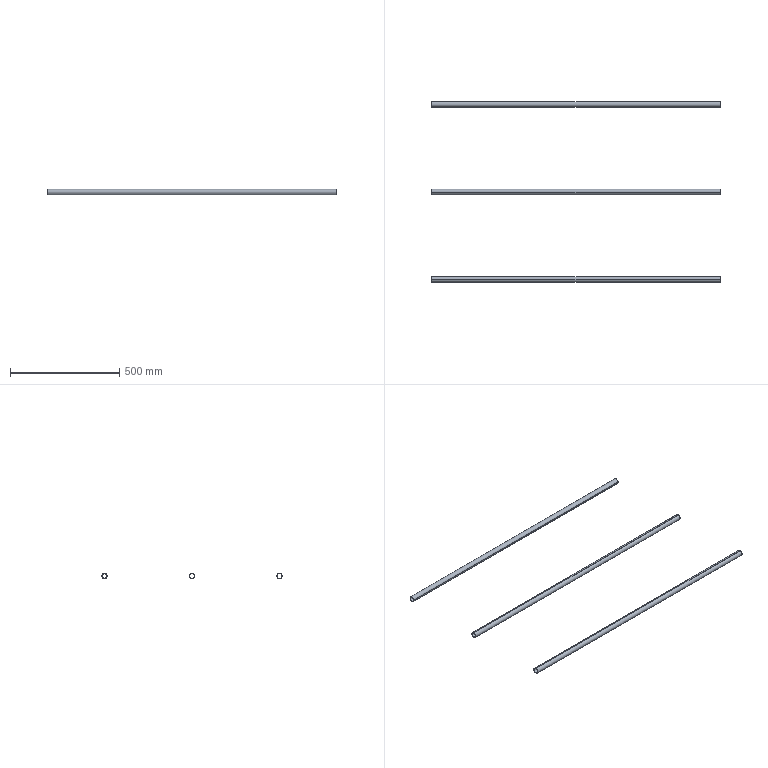Part | STEP file | 电柜护栏3栏杆_Default<As Machined> | 3 solids | 18 faces | box 1320 x 825 x 25 mm | volume 438535 mm3 | cylinder 12 | plane 6 | commonest cylinder face diameters 22 x6 25 x6
STEP:
#1=CARTESIAN_POINT('',(0.,0.,0.));
#2=DIRECTION('',(0.,0.,1.));
#3=DIRECTION('',(1.,0.,0.));
#4=AXIS2_PLACEMENT_3D('',#1,#2,#3);
#5=CARTESIAN_POINT('',(-1320.,0.,12.5));
#6=VERTEX_POINT('',#5);
#7=CARTESIAN_POINT('',(-1320.,0.,-12.5));
#8=VERTEX_POINT('',#7);
#9=CARTESIAN_POINT('',(-1320.,0.,0.));
#10=DIRECTION('',(-1.,0.,0.));
#11=DIRECTION('',(0.,-1.,0.));
#12=AXIS2_PLACEMENT_3D('',#9,#10,#11);
#13=CIRCLE('',#12,12.5);
#14=CARTESIAN_POINT('',(-1320.,0.,0.));
#15=DIRECTION('',(1.,0.,0.));
#16=DIRECTION('',(0.,0.,-1.));
#17=AXIS2_PLACEMENT_3D('',#14,#15,#16);
#18=CYLINDRICAL_SURFACE('',#17,12.5);
#19=CARTESIAN_POINT('',(4.712,0.));
#20=DIRECTION('',(-1.,0.));
#21=VECTOR('',#20,1.);
#22=LINE('',#19,#21);
#23=(GEOMETRIC_REPRESENTATION_CONTEXT(2)PARAMETRIC_REPRESENTATION_CONTEXT()REPRESENTATION_CONTEXT('',''));
#24=DEFINITIONAL_REPRESENTATION('',(#22),#23);
#25=PCURVE('',#18,#24);
#26=CARTESIAN_POINT('',(-1320.,0.,0.));
#27=DIRECTION('',(-1.,0.,0.));
#28=DIRECTION('',(0.,-1.,0.));
#29=AXIS2_PLACEMENT_3D('',#26,#27,#28);
#30=PLANE('',#29);
#31=CARTESIAN_POINT('',(0.,0.));
#32=DIRECTION('',(1.,0.));
#33=AXIS2_PLACEMENT_2D('',#31,#32);
#34=CIRCLE('',#33,12.5);
#35=(GEOMETRIC_REPRESENTATION_CONTEXT(2)PARAMETRIC_REPRESENTATION_CONTEXT()REPRESENTATION_CONTEXT('',''));
#36=DEFINITIONAL_REPRESENTATION('',(#34),#35);
#37=PCURVE('',#30,#36);
#38=SURFACE_CURVE('',#13,(#25,#37),.PCURVE_S1.);
#39=EDGE_CURVE('',#6,#8,#38,.T.);
#40=ORIENTED_EDGE('',*,*,#39,.F.);
#41=CARTESIAN_POINT('',(0.,0.,12.5));
#42=VERTEX_POINT('',#41);
#43=CARTESIAN_POINT('',(-1320.,0.,12.5));
#44=DIRECTION('',(1.,0.,0.));
#45=VECTOR('',#44,1.);
#46=LINE('',#43,#45);
#47=CARTESIAN_POINT('',(3.142,0.));
#48=DIRECTION('',(0.,1.));
#49=VECTOR('',#48,1.);
#50=LINE('',#47,#49);
#51=(GEOMETRIC_REPRESENTATION_CONTEXT(2)PARAMETRIC_REPRESENTATION_CONTEXT()REPRESENTATION_CONTEXT('',''));
#52=DEFINITIONAL_REPRESENTATION('',(#50),#51);
#53=PCURVE('',#18,#52);
#54=CARTESIAN_POINT('',(-1320.,0.,0.));
#55=DIRECTION('',(1.,0.,0.));
#56=DIRECTION('',(0.,0.,-1.));
#57=AXIS2_PLACEMENT_3D('',#54,#55,#56);
#58=CYLINDRICAL_SURFACE('',#57,12.5);
#59=CARTESIAN_POINT('',(3.142,0.));
#60=DIRECTION('',(0.,1.));
#61=VECTOR('',#60,1.);
#62=LINE('',#59,#61);
#63=(GEOMETRIC_REPRESENTATION_CONTEXT(2)PARAMETRIC_REPRESENTATION_CONTEXT()REPRESENTATION_CONTEXT('',''));
#64=DEFINITIONAL_REPRESENTATION('',(#62),#63);
#65=PCURVE('',#58,#64);
#66=SURFACE_CURVE('',#46,(#53,#65),.PCURVE_S1.);
#67=EDGE_CURVE('',#6,#42,#66,.T.);
#68=ORIENTED_EDGE('',*,*,#67,.T.);
#69=CARTESIAN_POINT('',(0.,0.,-12.5));
#70=VERTEX_POINT('',#69);
#71=CARTESIAN_POINT('',(0.,0.,0.));
#72=DIRECTION('',(-1.,0.,0.));
#73=DIRECTION('',(0.,-1.,0.));
#74=AXIS2_PLACEMENT_3D('',#71,#72,#73);
#75=CIRCLE('',#74,12.5);
#76=CARTESIAN_POINT('',(4.712,1320.));
#77=DIRECTION('',(-1.,0.));
#78=VECTOR('',#77,1.);
#79=LINE('',#76,#78);
#80=(GEOMETRIC_REPRESENTATION_CONTEXT(2)PARAMETRIC_REPRESENTATION_CONTEXT()REPRESENTATION_CONTEXT('',''));
#81=DEFINITIONAL_REPRESENTATION('',(#79),#80);
#82=PCURVE('',#18,#81);
#83=CARTESIAN_POINT('',(0.,0.,0.));
#84=DIRECTION('',(-1.,0.,0.));
#85=DIRECTION('',(0.,-1.,0.));
#86=AXIS2_PLACEMENT_3D('',#83,#84,#85);
#87=PLANE('',#86);
#88=CARTESIAN_POINT('',(0.,0.));
#89=DIRECTION('',(1.,0.));
#90=AXIS2_PLACEMENT_2D('',#88,#89);
#91=CIRCLE('',#90,12.5);
#92=(GEOMETRIC_REPRESENTATION_CONTEXT(2)PARAMETRIC_REPRESENTATION_CONTEXT()REPRESENTATION_CONTEXT('',''));
#93=DEFINITIONAL_REPRESENTATION('',(#91),#92);
#94=PCURVE('',#87,#93);
#95=SURFACE_CURVE('',#75,(#82,#94),.PCURVE_S1.);
#96=EDGE_CURVE('',#42,#70,#95,.T.);
#97=ORIENTED_EDGE('',*,*,#96,.T.);
#98=CARTESIAN_POINT('',(-1320.,0.,-12.5));
#99=DIRECTION('',(1.,0.,0.));
#100=VECTOR('',#99,1.);
#101=LINE('',#98,#100);
#102=CARTESIAN_POINT('',(0.,0.));
#103=DIRECTION('',(0.,1.));
#104=VECTOR('',#103,1.);
#105=LINE('',#102,#104);
#106=(GEOMETRIC_REPRESENTATION_CONTEXT(2)PARAMETRIC_REPRESENTATION_CONTEXT()REPRESENTATION_CONTEXT('',''));
#107=DEFINITIONAL_REPRESENTATION('',(#105),#106);
#108=PCURVE('',#18,#107);
#109=CARTESIAN_POINT('',(6.283,0.));
#110=DIRECTION('',(0.,1.));
#111=VECTOR('',#110,1.);
#112=LINE('',#109,#111);
#113=(GEOMETRIC_REPRESENTATION_CONTEXT(2)PARAMETRIC_REPRESENTATION_CONTEXT()REPRESENTATION_CONTEXT('',''));
#114=DEFINITIONAL_REPRESENTATION('',(#112),#113);
#115=PCURVE('',#58,#114);
#116=SURFACE_CURVE('',#101,(#108,#115),.PCURVE_S1.);
#117=EDGE_CURVE('',#8,#70,#116,.T.);
#118=ORIENTED_EDGE('',*,*,#117,.F.);
#119=EDGE_LOOP('',(#40,#68,#97,#118));
#120=FACE_BOUND('',#119,.T.);
#121=ADVANCED_FACE('',(#120),#18,.T.);
#122=CARTESIAN_POINT('',(-1320.,0.,-11.));
#123=VERTEX_POINT('',#122);
#124=CARTESIAN_POINT('',(0.,0.,-11.));
#125=VERTEX_POINT('',#124);
#126=CARTESIAN_POINT('',(-1320.,0.,-11.));
#127=DIRECTION('',(1.,0.,0.));
#128=VECTOR('',#127,1.);
#129=LINE('',#126,#128);
#130=CARTESIAN_POINT('',(-1320.,0.,0.));
#131=DIRECTION('',(1.,0.,0.));
#132=DIRECTION('',(0.,0.,-1.));
#133=AXIS2_PLACEMENT_3D('',#130,#131,#132);
#134=CYLINDRICAL_SURFACE('',#133,11.);
#135=CARTESIAN_POINT('',(6.283,0.));
#136=DIRECTION('',(0.,1.));
#137=VECTOR('',#136,1.);
#138=LINE('',#135,#137);
#139=(GEOMETRIC_REPRESENTATION_CONTEXT(2)PARAMETRIC_REPRESENTATION_CONTEXT()REPRESENTATION_CONTEXT('',''));
#140=DEFINITIONAL_REPRESENTATION('',(#138),#139);
#141=PCURVE('',#134,#140);
#142=CARTESIAN_POINT('',(-1320.,0.,0.));
#143=DIRECTION('',(1.,0.,0.));
#144=DIRECTION('',(0.,0.,-1.));
#145=AXIS2_PLACEMENT_3D('',#142,#143,#144);
#146=CYLINDRICAL_SURFACE('',#145,11.);
#147=CARTESIAN_POINT('',(0.,0.));
#148=DIRECTION('',(0.,1.));
#149=VECTOR('',#148,1.);
#150=LINE('',#147,#149);
#151=(GEOMETRIC_REPRESENTATION_CONTEXT(2)PARAMETRIC_REPRESENTATION_CONTEXT()REPRESENTATION_CONTEXT('',''));
#152=DEFINITIONAL_REPRESENTATION('',(#150),#151);
#153=PCURVE('',#146,#152);
#154=SURFACE_CURVE('',#129,(#141,#153),.PCURVE_S1.);
#155=EDGE_CURVE('',#123,#125,#154,.T.);
#156=ORIENTED_EDGE('',*,*,#155,.T.);
#157=CARTESIAN_POINT('',(0.,0.,11.));
#158=VERTEX_POINT('',#157);
#159=CARTESIAN_POINT('',(0.,0.,0.));
#160=DIRECTION('',(-1.,0.,0.));
#161=DIRECTION('',(0.,-1.,0.));
#162=AXIS2_PLACEMENT_3D('',#159,#160,#161);
#163=CIRCLE('',#162,11.);
#164=CARTESIAN_POINT('',(10.996,1320.));
#165=DIRECTION('',(-1.,0.));
#166=VECTOR('',#165,1.);
#167=LINE('',#164,#166);
#168=(GEOMETRIC_REPRESENTATION_CONTEXT(2)PARAMETRIC_REPRESENTATION_CONTEXT()REPRESENTATION_CONTEXT('',''));
#169=DEFINITIONAL_REPRESENTATION('',(#167),#168);
#170=PCURVE('',#134,#169);
#171=CARTESIAN_POINT('',(0.,0.));
#172=DIRECTION('',(1.,0.));
#173=AXIS2_PLACEMENT_2D('',#171,#172);
#174=CIRCLE('',#173,11.);
#175=(GEOMETRIC_REPRESENTATION_CONTEXT(2)PARAMETRIC_REPRESENTATION_CONTEXT()REPRESENTATION_CONTEXT('',''));
#176=DEFINITIONAL_REPRESENTATION('',(#174),#175);
#177=PCURVE('',#87,#176);
#178=SURFACE_CURVE('',#163,(#170,#177),.PCURVE_S1.);
#179=EDGE_CURVE('',#125,#158,#178,.T.);
#180=ORIENTED_EDGE('',*,*,#179,.T.);
#181=CARTESIAN_POINT('',(-1320.,0.,11.));
#182=VERTEX_POINT('',#181);
#183=CARTESIAN_POINT('',(-1320.,0.,11.));
#184=DIRECTION('',(1.,0.,0.));
#185=VECTOR('',#184,1.);
#186=LINE('',#183,#185);
#187=CARTESIAN_POINT('',(3.142,0.));
#188=DIRECTION('',(0.,1.));
#189=VECTOR('',#188,1.);
#190=LINE('',#187,#189);
#191=(GEOMETRIC_REPRESENTATION_CONTEXT(2)PARAMETRIC_REPRESENTATION_CONTEXT()REPRESENTATION_CONTEXT('',''));
#192=DEFINITIONAL_REPRESENTATION('',(#190),#191);
#193=PCURVE('',#134,#192);
#194=CARTESIAN_POINT('',(3.142,0.));
#195=DIRECTION('',(0.,1.));
#196=VECTOR('',#195,1.);
#197=LINE('',#194,#196);
#198=(GEOMETRIC_REPRESENTATION_CONTEXT(2)PARAMETRIC_REPRESENTATION_CONTEXT()REPRESENTATION_CONTEXT('',''));
#199=DEFINITIONAL_REPRESENTATION('',(#197),#198);
#200=PCURVE('',#146,#199);
#201=SURFACE_CURVE('',#186,(#193,#200),.PCURVE_S1.);
#202=EDGE_CURVE('',#182,#158,#201,.T.);
#203=ORIENTED_EDGE('',*,*,#202,.F.);
#204=CARTESIAN_POINT('',(-1320.,0.,0.));
#205=DIRECTION('',(-1.,0.,0.));
#206=DIRECTION('',(0.,-1.,0.));
#207=AXIS2_PLACEMENT_3D('',#204,#205,#206);
#208=CIRCLE('',#207,11.);
#209=CARTESIAN_POINT('',(10.996,0.));
#210=DIRECTION('',(-1.,0.));
#211=VECTOR('',#210,1.);
#212=LINE('',#209,#211);
#213=(GEOMETRIC_REPRESENTATION_CONTEXT(2)PARAMETRIC_REPRESENTATION_CONTEXT()REPRESENTATION_CONTEXT('',''));
#214=DEFINITIONAL_REPRESENTATION('',(#212),#213);
#215=PCURVE('',#134,#214);
#216=CARTESIAN_POINT('',(0.,0.));
#217=DIRECTION('',(1.,0.));
#218=AXIS2_PLACEMENT_2D('',#216,#217);
#219=CIRCLE('',#218,11.);
#220=(GEOMETRIC_REPRESENTATION_CONTEXT(2)PARAMETRIC_REPRESENTATION_CONTEXT()REPRESENTATION_CONTEXT('',''));
#221=DEFINITIONAL_REPRESENTATION('',(#219),#220);
#222=PCURVE('',#30,#221);
#223=SURFACE_CURVE('',#208,(#215,#222),.PCURVE_S1.);
#224=EDGE_CURVE('',#123,#182,#223,.T.);
#225=ORIENTED_EDGE('',*,*,#224,.F.);
#226=EDGE_LOOP('',(#156,#180,#203,#225));
#227=FACE_BOUND('',#226,.F.);
#228=ADVANCED_FACE('',(#227),#134,.F.);
#229=CARTESIAN_POINT('',(0.,0.,0.));
#230=DIRECTION('',(-1.,0.,0.));
#231=DIRECTION('',(0.,-1.,0.));
#232=AXIS2_PLACEMENT_3D('',#229,#230,#231);
#233=CIRCLE('',#232,11.);
#234=CARTESIAN_POINT('',(4.712,1320.));
#235=DIRECTION('',(-1.,0.));
#236=VECTOR('',#235,1.);
#237=LINE('',#234,#236);
#238=(GEOMETRIC_REPRESENTATION_CONTEXT(2)PARAMETRIC_REPRESENTATION_CONTEXT()REPRESENTATION_CONTEXT('',''));
#239=DEFINITIONAL_REPRESENTATION('',(#237),#238);
#240=PCURVE('',#146,#239);
#241=CARTESIAN_POINT('',(0.,0.));
#242=DIRECTION('',(1.,0.));
#243=AXIS2_PLACEMENT_2D('',#241,#242);
#244=CIRCLE('',#243,11.);
#245=(GEOMETRIC_REPRESENTATION_CONTEXT(2)PARAMETRIC_REPRESENTATION_CONTEXT()REPRESENTATION_CONTEXT('',''));
#246=DEFINITIONAL_REPRESENTATION('',(#244),#245);
#247=PCURVE('',#87,#246);
#248=SURFACE_CURVE('',#233,(#240,#247),.PCURVE_S1.);
#249=EDGE_CURVE('',#158,#125,#248,.T.);
#250=ORIENTED_EDGE('',*,*,#249,.T.);
#251=ORIENTED_EDGE('',*,*,#155,.F.);
#252=CARTESIAN_POINT('',(-1320.,0.,0.));
#253=DIRECTION('',(-1.,0.,0.));
#254=DIRECTION('',(0.,-1.,0.));
#255=AXIS2_PLACEMENT_3D('',#252,#253,#254);
#256=CIRCLE('',#255,11.);
#257=CARTESIAN_POINT('',(4.712,0.));
#258=DIRECTION('',(-1.,0.));
#259=VECTOR('',#258,1.);
#260=LINE('',#257,#259);
#261=(GEOMETRIC_REPRESENTATION_CONTEXT(2)PARAMETRIC_REPRESENTATION_CONTEXT()REPRESENTATION_CONTEXT('',''));
#262=DEFINITIONAL_REPRESENTATION('',(#260),#261);
#263=PCURVE('',#146,#262);
#264=CARTESIAN_POINT('',(0.,0.));
#265=DIRECTION('',(1.,0.));
#266=AXIS2_PLACEMENT_2D('',#264,#265);
#267=CIRCLE('',#266,11.);
#268=(GEOMETRIC_REPRESENTATION_CONTEXT(2)PARAMETRIC_REPRESENTATION_CONTEXT()REPRESENTATION_CONTEXT('',''));
#269=DEFINITIONAL_REPRESENTATION('',(#267),#268);
#270=PCURVE('',#30,#269);
#271=SURFACE_CURVE('',#256,(#263,#270),.PCURVE_S1.);
#272=EDGE_CURVE('',#182,#123,#271,.T.);
#273=ORIENTED_EDGE('',*,*,#272,.F.);
#274=ORIENTED_EDGE('',*,*,#202,.T.);
#275=EDGE_LOOP('',(#250,#251,#273,#274));
#276=FACE_BOUND('',#275,.F.);
#277=ADVANCED_FACE('',(#276),#146,.F.);
#278=ORIENTED_EDGE('',*,*,#67,.F.);
#279=CARTESIAN_POINT('',(-1320.,0.,0.));
#280=DIRECTION('',(-1.,0.,0.));
#281=DIRECTION('',(0.,-1.,0.));
#282=AXIS2_PLACEMENT_3D('',#279,#280,#281);
#283=CIRCLE('',#282,12.5);
#284=CARTESIAN_POINT('',(10.996,0.));
#285=DIRECTION('',(-1.,0.));
#286=VECTOR('',#285,1.);
#287=LINE('',#284,#286);
#288=(GEOMETRIC_REPRESENTATION_CONTEXT(2)PARAMETRIC_REPRESENTATION_CONTEXT()REPRESENTATION_CONTEXT('',''));
#289=DEFINITIONAL_REPRESENTATION('',(#287),#288);
#290=PCURVE('',#58,#289);
#291=CARTESIAN_POINT('',(0.,0.));
#292=DIRECTION('',(1.,0.));
#293=AXIS2_PLACEMENT_2D('',#291,#292);
#294=CIRCLE('',#293,12.5);
#295=(GEOMETRIC_REPRESENTATION_CONTEXT(2)PARAMETRIC_REPRESENTATION_CONTEXT()REPRESENTATION_CONTEXT('',''));
#296=DEFINITIONAL_REPRESENTATION('',(#294),#295);
#297=PCURVE('',#30,#296);
#298=SURFACE_CURVE('',#283,(#290,#297),.PCURVE_S1.);
#299=EDGE_CURVE('',#8,#6,#298,.T.);
#300=ORIENTED_EDGE('',*,*,#299,.F.);
#301=ORIENTED_EDGE('',*,*,#117,.T.);
#302=CARTESIAN_POINT('',(0.,0.,0.));
#303=DIRECTION('',(-1.,0.,0.));
#304=DIRECTION('',(0.,-1.,0.));
#305=AXIS2_PLACEMENT_3D('',#302,#303,#304);
#306=CIRCLE('',#305,12.5);
#307=CARTESIAN_POINT('',(10.996,1320.));
#308=DIRECTION('',(-1.,0.));
#309=VECTOR('',#308,1.);
#310=LINE('',#307,#309);
#311=(GEOMETRIC_REPRESENTATION_CONTEXT(2)PARAMETRIC_REPRESENTATION_CONTEXT()REPRESENTATION_CONTEXT('',''));
#312=DEFINITIONAL_REPRESENTATION('',(#310),#311);
#313=PCURVE('',#58,#312);
#314=CARTESIAN_POINT('',(0.,0.));
#315=DIRECTION('',(1.,0.));
#316=AXIS2_PLACEMENT_2D('',#314,#315);
#317=CIRCLE('',#316,12.5);
#318=(GEOMETRIC_REPRESENTATION_CONTEXT(2)PARAMETRIC_REPRESENTATION_CONTEXT()REPRESENTATION_CONTEXT('',''));
#319=DEFINITIONAL_REPRESENTATION('',(#317),#318);
#320=PCURVE('',#87,#319);
#321=SURFACE_CURVE('',#306,(#313,#320),.PCURVE_S1.);
#322=EDGE_CURVE('',#70,#42,#321,.T.);
#323=ORIENTED_EDGE('',*,*,#322,.T.);
#324=EDGE_LOOP('',(#278,#300,#301,#323));
#325=FACE_BOUND('',#324,.T.);
#326=ADVANCED_FACE('',(#325),#58,.T.);
#327=ORIENTED_EDGE('',*,*,#224,.F.);
#328=ORIENTED_EDGE('',*,*,#272,.F.);
#329=EDGE_LOOP('',(#327,#328));
#330=FACE_BOUND('',#329,.T.);
#331=ORIENTED_EDGE('',*,*,#299,.T.);
#332=ORIENTED_EDGE('',*,*,#39,.T.);
#333=EDGE_LOOP('',(#331,#332));
#334=FACE_BOUND('',#333,.T.);
#335=ADVANCED_FACE('',(#330,#334),#30,.T.);
#336=ORIENTED_EDGE('',*,*,#179,.T.);
#337=ORIENTED_EDGE('',*,*,#249,.T.);
#338=EDGE_LOOP('',(#336,#337));
#339=FACE_BOUND('',#338,.T.);
#340=ORIENTED_EDGE('',*,*,#322,.F.);
#341=ORIENTED_EDGE('',*,*,#96,.F.);
#342=EDGE_LOOP('',(#340,#341));
#343=FACE_BOUND('',#342,.T.);
#344=ADVANCED_FACE('',(#339,#343),#87,.F.);
#345=CLOSED_SHELL('',(#121,#228,#277,#326,#335,#344));
#346=MANIFOLD_SOLID_BREP('',#345);
#347=CARTESIAN_POINT('',(-1320.,787.5,0.));
#348=VERTEX_POINT('',#347);
#349=CARTESIAN_POINT('',(-1320.,812.5,0.));
#350=VERTEX_POINT('',#349);
#351=CARTESIAN_POINT('',(-1320.,800.,0.));
#352=DIRECTION('',(-1.,0.,0.));
#353=DIRECTION('',(0.,-1.,0.));
#354=AXIS2_PLACEMENT_3D('',#351,#352,#353);
#355=CIRCLE('',#354,12.5);
#356=CARTESIAN_POINT('',(-1320.,800.,0.));
#357=DIRECTION('',(1.,0.,0.));
#358=DIRECTION('',(0.,1.,0.));
#359=AXIS2_PLACEMENT_3D('',#356,#357,#358);
#360=CYLINDRICAL_SURFACE('',#359,12.5);
#361=CARTESIAN_POINT('',(3.142,0.));
#362=DIRECTION('',(-1.,0.));
#363=VECTOR('',#362,1.);
#364=LINE('',#361,#363);
#365=(GEOMETRIC_REPRESENTATION_CONTEXT(2)PARAMETRIC_REPRESENTATION_CONTEXT()REPRESENTATION_CONTEXT('',''));
#366=DEFINITIONAL_REPRESENTATION('',(#364),#365);
#367=PCURVE('',#360,#366);
#368=CARTESIAN_POINT('',(-1320.,800.,0.));
#369=DIRECTION('',(-1.,0.,0.));
#370=DIRECTION('',(0.,-1.,0.));
#371=AXIS2_PLACEMENT_3D('',#368,#369,#370);
#372=PLANE('',#371);
#373=CARTESIAN_POINT('',(0.,0.));
#374=DIRECTION('',(1.,0.));
#375=AXIS2_PLACEMENT_2D('',#373,#374);
#376=CIRCLE('',#375,12.5);
#377=(GEOMETRIC_REPRESENTATION_CONTEXT(2)PARAMETRIC_REPRESENTATION_CONTEXT()REPRESENTATION_CONTEXT('',''));
#378=DEFINITIONAL_REPRESENTATION('',(#376),#377);
#379=PCURVE('',#372,#378);
#380=SURFACE_CURVE('',#355,(#367,#379),.PCURVE_S1.);
#381=EDGE_CURVE('',#348,#350,#380,.T.);
#382=ORIENTED_EDGE('',*,*,#381,.F.);
#383=CARTESIAN_POINT('',(0.,787.5,0.));
#384=VERTEX_POINT('',#383);
#385=CARTESIAN_POINT('',(-1320.,787.5,0.));
#386=DIRECTION('',(1.,0.,0.));
#387=VECTOR('',#386,1.);
#388=LINE('',#385,#387);
#389=CARTESIAN_POINT('',(3.142,0.));
#390=DIRECTION('',(0.,1.));
#391=VECTOR('',#390,1.);
#392=LINE('',#389,#391);
#393=(GEOMETRIC_REPRESENTATION_CONTEXT(2)PARAMETRIC_REPRESENTATION_CONTEXT()REPRESENTATION_CONTEXT('',''));
#394=DEFINITIONAL_REPRESENTATION('',(#392),#393);
#395=PCURVE('',#360,#394);
#396=CARTESIAN_POINT('',(-1320.,800.,0.));
#397=DIRECTION('',(1.,0.,0.));
#398=DIRECTION('',(0.,1.,0.));
#399=AXIS2_PLACEMENT_3D('',#396,#397,#398);
#400=CYLINDRICAL_SURFACE('',#399,12.5);
#401=CARTESIAN_POINT('',(3.142,0.));
#402=DIRECTION('',(0.,1.));
#403=VECTOR('',#402,1.);
#404=LINE('',#401,#403);
#405=(GEOMETRIC_REPRESENTATION_CONTEXT(2)PARAMETRIC_REPRESENTATION_CONTEXT()REPRESENTATION_CONTEXT('',''));
#406=DEFINITIONAL_REPRESENTATION('',(#404),#405);
#407=PCURVE('',#400,#406);
#408=SURFACE_CURVE('',#388,(#395,#407),.PCURVE_S1.);
#409=EDGE_CURVE('',#348,#384,#408,.T.);
#410=ORIENTED_EDGE('',*,*,#409,.T.);
#411=CARTESIAN_POINT('',(0.,812.5,0.));
#412=VERTEX_POINT('',#411);
#413=CARTESIAN_POINT('',(0.,800.,0.));
#414=DIRECTION('',(-1.,0.,0.));
#415=DIRECTION('',(0.,-1.,0.));
#416=AXIS2_PLACEMENT_3D('',#413,#414,#415);
#417=CIRCLE('',#416,12.5);
#418=CARTESIAN_POINT('',(3.142,1320.));
#419=DIRECTION('',(-1.,0.));
#420=VECTOR('',#419,1.);
#421=LINE('',#418,#420);
#422=(GEOMETRIC_REPRESENTATION_CONTEXT(2)PARAMETRIC_REPRESENTATION_CONTEXT()REPRESENTATION_CONTEXT('',''));
#423=DEFINITIONAL_REPRESENTATION('',(#421),#422);
#424=PCURVE('',#360,#423);
#425=CARTESIAN_POINT('',(0.,800.,0.));
#426=DIRECTION('',(-1.,0.,0.));
#427=DIRECTION('',(0.,-1.,0.));
#428=AXIS2_PLACEMENT_3D('',#425,#426,#427);
#429=PLANE('',#428);
#430=CARTESIAN_POINT('',(0.,0.));
#431=DIRECTION('',(1.,0.));
#432=AXIS2_PLACEMENT_2D('',#430,#431);
#433=CIRCLE('',#432,12.5);
#434=(GEOMETRIC_REPRESENTATION_CONTEXT(2)PARAMETRIC_REPRESENTATION_CONTEXT()REPRESENTATION_CONTEXT('',''));
#435=DEFINITIONAL_REPRESENTATION('',(#433),#434);
#436=PCURVE('',#429,#435);
#437=SURFACE_CURVE('',#417,(#424,#436),.PCURVE_S1.);
#438=EDGE_CURVE('',#384,#412,#437,.T.);
#439=ORIENTED_EDGE('',*,*,#438,.T.);
#440=CARTESIAN_POINT('',(-1320.,812.5,0.));
#441=DIRECTION('',(1.,0.,0.));
#442=VECTOR('',#441,1.);
#443=LINE('',#440,#442);
#444=CARTESIAN_POINT('',(0.,0.));
#445=DIRECTION('',(0.,1.));
#446=VECTOR('',#445,1.);
#447=LINE('',#444,#446);
#448=(GEOMETRIC_REPRESENTATION_CONTEXT(2)PARAMETRIC_REPRESENTATION_CONTEXT()REPRESENTATION_CONTEXT('',''));
#449=DEFINITIONAL_REPRESENTATION('',(#447),#448);
#450=PCURVE('',#360,#449);
#451=CARTESIAN_POINT('',(6.283,0.));
#452=DIRECTION('',(0.,1.));
#453=VECTOR('',#452,1.);
#454=LINE('',#451,#453);
#455=(GEOMETRIC_REPRESENTATION_CONTEXT(2)PARAMETRIC_REPRESENTATION_CONTEXT()REPRESENTATION_CONTEXT('',''));
#456=DEFINITIONAL_REPRESENTATION('',(#454),#455);
#457=PCURVE('',#400,#456);
#458=SURFACE_CURVE('',#443,(#450,#457),.PCURVE_S1.);
#459=EDGE_CURVE('',#350,#412,#458,.T.);
#460=ORIENTED_EDGE('',*,*,#459,.F.);
#461=EDGE_LOOP('',(#382,#410,#439,#460));
#462=FACE_BOUND('',#461,.T.);
#463=ADVANCED_FACE('',(#462),#360,.T.);
#464=CARTESIAN_POINT('',(-1320.,811.,0.));
#465=VERTEX_POINT('',#464);
#466=CARTESIAN_POINT('',(0.,811.,0.));
#467=VERTEX_POINT('',#466);
#468=CARTESIAN_POINT('',(-1320.,811.,0.));
#469=DIRECTION('',(1.,0.,0.));
#470=VECTOR('',#469,1.);
#471=LINE('',#468,#470);
#472=CARTESIAN_POINT('',(-1320.,800.,0.));
#473=DIRECTION('',(1.,0.,0.));
#474=DIRECTION('',(0.,1.,0.));
#475=AXIS2_PLACEMENT_3D('',#472,#473,#474);
#476=CYLINDRICAL_SURFACE('',#475,11.);
#477=CARTESIAN_POINT('',(6.283,0.));
#478=DIRECTION('',(0.,1.));
#479=VECTOR('',#478,1.);
#480=LINE('',#477,#479);
#481=(GEOMETRIC_REPRESENTATION_CONTEXT(2)PARAMETRIC_REPRESENTATION_CONTEXT()REPRESENTATION_CONTEXT('',''));
#482=DEFINITIONAL_REPRESENTATION('',(#480),#481);
#483=PCURVE('',#476,#482);
#484=CARTESIAN_POINT('',(-1320.,800.,0.));
#485=DIRECTION('',(1.,0.,0.));
#486=DIRECTION('',(0.,1.,0.));
#487=AXIS2_PLACEMENT_3D('',#484,#485,#486);
#488=CYLINDRICAL_SURFACE('',#487,11.);
#489=CARTESIAN_POINT('',(0.,0.));
#490=DIRECTION('',(0.,1.));
#491=VECTOR('',#490,1.);
#492=LINE('',#489,#491);
#493=(GEOMETRIC_REPRESENTATION_CONTEXT(2)PARAMETRIC_REPRESENTATION_CONTEXT()REPRESENTATION_CONTEXT('',''));
#494=DEFINITIONAL_REPRESENTATION('',(#492),#493);
#495=PCURVE('',#488,#494);
#496=SURFACE_CURVE('',#471,(#483,#495),.PCURVE_S1.);
#497=EDGE_CURVE('',#465,#467,#496,.T.);
#498=ORIENTED_EDGE('',*,*,#497,.T.);
#499=CARTESIAN_POINT('',(0.,789.,0.));
#500=VERTEX_POINT('',#499);
#501=CARTESIAN_POINT('',(0.,800.,0.));
#502=DIRECTION('',(-1.,0.,0.));
#503=DIRECTION('',(0.,-1.,0.));
#504=AXIS2_PLACEMENT_3D('',#501,#502,#503);
#505=CIRCLE('',#504,11.);
#506=CARTESIAN_POINT('',(9.425,1320.));
#507=DIRECTION('',(-1.,0.));
#508=VECTOR('',#507,1.);
#509=LINE('',#506,#508);
#510=(GEOMETRIC_REPRESENTATION_CONTEXT(2)PARAMETRIC_REPRESENTATION_CONTEXT()REPRESENTATION_CONTEXT('',''));
#511=DEFINITIONAL_REPRESENTATION('',(#509),#510);
#512=PCURVE('',#476,#511);
#513=CARTESIAN_POINT('',(0.,0.));
#514=DIRECTION('',(1.,0.));
#515=AXIS2_PLACEMENT_2D('',#513,#514);
#516=CIRCLE('',#515,11.);
#517=(GEOMETRIC_REPRESENTATION_CONTEXT(2)PARAMETRIC_REPRESENTATION_CONTEXT()REPRESENTATION_CONTEXT('',''));
#518=DEFINITIONAL_REPRESENTATION('',(#516),#517);
#519=PCURVE('',#429,#518);
#520=SURFACE_CURVE('',#505,(#512,#519),.PCURVE_S1.);
#521=EDGE_CURVE('',#467,#500,#520,.T.);
#522=ORIENTED_EDGE('',*,*,#521,.T.);
#523=CARTESIAN_POINT('',(-1320.,789.,0.));
#524=VERTEX_POINT('',#523);
#525=CARTESIAN_POINT('',(-1320.,789.,0.));
#526=DIRECTION('',(1.,0.,0.));
#527=VECTOR('',#526,1.);
#528=LINE('',#525,#527);
#529=CARTESIAN_POINT('',(3.142,0.));
#530=DIRECTION('',(0.,1.));
#531=VECTOR('',#530,1.);
#532=LINE('',#529,#531);
#533=(GEOMETRIC_REPRESENTATION_CONTEXT(2)PARAMETRIC_REPRESENTATION_CONTEXT()REPRESENTATION_CONTEXT('',''));
#534=DEFINITIONAL_REPRESENTATION('',(#532),#533);
#535=PCURVE('',#476,#534);
#536=CARTESIAN_POINT('',(3.142,0.));
#537=DIRECTION('',(0.,1.));
#538=VECTOR('',#537,1.);
#539=LINE('',#536,#538);
#540=(GEOMETRIC_REPRESENTATION_CONTEXT(2)PARAMETRIC_REPRESENTATION_CONTEXT()REPRESENTATION_CONTEXT('',''));
#541=DEFINITIONAL_REPRESENTATION('',(#539),#540);
#542=PCURVE('',#488,#541);
#543=SURFACE_CURVE('',#528,(#535,#542),.PCURVE_S1.);
#544=EDGE_CURVE('',#524,#500,#543,.T.);
#545=ORIENTED_EDGE('',*,*,#544,.F.);
#546=CARTESIAN_POINT('',(-1320.,800.,0.));
#547=DIRECTION('',(-1.,0.,0.));
#548=DIRECTION('',(0.,-1.,0.));
#549=AXIS2_PLACEMENT_3D('',#546,#547,#548);
#550=CIRCLE('',#549,11.);
#551=CARTESIAN_POINT('',(9.425,0.));
#552=DIRECTION('',(-1.,0.));
#553=VECTOR('',#552,1.);
#554=LINE('',#551,#553);
#555=(GEOMETRIC_REPRESENTATION_CONTEXT(2)PARAMETRIC_REPRESENTATION_CONTEXT()REPRESENTATION_CONTEXT('',''));
#556=DEFINITIONAL_REPRESENTATION('',(#554),#555);
#557=PCURVE('',#476,#556);
#558=CARTESIAN_POINT('',(0.,0.));
#559=DIRECTION('',(1.,0.));
#560=AXIS2_PLACEMENT_2D('',#558,#559);
#561=CIRCLE('',#560,11.);
#562=(GEOMETRIC_REPRESENTATION_CONTEXT(2)PARAMETRIC_REPRESENTATION_CONTEXT()REPRESENTATION_CONTEXT('',''));
#563=DEFINITIONAL_REPRESENTATION('',(#561),#562);
#564=PCURVE('',#372,#563);
#565=SURFACE_CURVE('',#550,(#557,#564),.PCURVE_S1.);
#566=EDGE_CURVE('',#465,#524,#565,.T.);
#567=ORIENTED_EDGE('',*,*,#566,.F.);
#568=EDGE_LOOP('',(#498,#522,#545,#567));
#569=FACE_BOUND('',#568,.F.);
#570=ADVANCED_FACE('',(#569),#476,.F.);
#571=CARTESIAN_POINT('',(0.,800.,0.));
#572=DIRECTION('',(-1.,0.,0.));
#573=DIRECTION('',(0.,-1.,0.));
#574=AXIS2_PLACEMENT_3D('',#571,#572,#573);
#575=CIRCLE('',#574,11.);
#576=CARTESIAN_POINT('',(3.142,1320.));
#577=DIRECTION('',(-1.,0.));
#578=VECTOR('',#577,1.);
#579=LINE('',#576,#578);
#580=(GEOMETRIC_REPRESENTATION_CONTEXT(2)PARAMETRIC_REPRESENTATION_CONTEXT()REPRESENTATION_CONTEXT('',''));
#581=DEFINITIONAL_REPRESENTATION('',(#579),#580);
#582=PCURVE('',#488,#581);
#583=CARTESIAN_POINT('',(0.,0.));
#584=DIRECTION('',(1.,0.));
#585=AXIS2_PLACEMENT_2D('',#583,#584);
#586=CIRCLE('',#585,11.);
#587=(GEOMETRIC_REPRESENTATION_CONTEXT(2)PARAMETRIC_REPRESENTATION_CONTEXT()REPRESENTATION_CONTEXT('',''));
#588=DEFINITIONAL_REPRESENTATION('',(#586),#587);
#589=PCURVE('',#429,#588);
#590=SURFACE_CURVE('',#575,(#582,#589),.PCURVE_S1.);
#591=EDGE_CURVE('',#500,#467,#590,.T.);
#592=ORIENTED_EDGE('',*,*,#591,.T.);
#593=ORIENTED_EDGE('',*,*,#497,.F.);
#594=CARTESIAN_POINT('',(-1320.,800.,0.));
#595=DIRECTION('',(-1.,0.,0.));
#596=DIRECTION('',(0.,-1.,0.));
#597=AXIS2_PLACEMENT_3D('',#594,#595,#596);
#598=CIRCLE('',#597,11.);
#599=CARTESIAN_POINT('',(3.142,0.));
#600=DIRECTION('',(-1.,0.));
#601=VECTOR('',#600,1.);
#602=LINE('',#599,#601);
#603=(GEOMETRIC_REPRESENTATION_CONTEXT(2)PARAMETRIC_REPRESENTATION_CONTEXT()REPRESENTATION_CONTEXT('',''));
#604=DEFINITIONAL_REPRESENTATION('',(#602),#603);
#605=PCURVE('',#488,#604);
#606=CARTESIAN_POINT('',(0.,0.));
#607=DIRECTION('',(1.,0.));
#608=AXIS2_PLACEMENT_2D('',#606,#607);
#609=CIRCLE('',#608,11.);
#610=(GEOMETRIC_REPRESENTATION_CONTEXT(2)PARAMETRIC_REPRESENTATION_CONTEXT()REPRESENTATION_CONTEXT('',''));
#611=DEFINITIONAL_REPRESENTATION('',(#609),#610);
#612=PCURVE('',#372,#611);
#613=SURFACE_CURVE('',#598,(#605,#612),.PCURVE_S1.);
#614=EDGE_CURVE('',#524,#465,#613,.T.);
#615=ORIENTED_EDGE('',*,*,#614,.F.);
#616=ORIENTED_EDGE('',*,*,#544,.T.);
#617=EDGE_LOOP('',(#592,#593,#615,#616));
#618=FACE_BOUND('',#617,.F.);
#619=ADVANCED_FACE('',(#618),#488,.F.);
#620=ORIENTED_EDGE('',*,*,#409,.F.);
#621=CARTESIAN_POINT('',(-1320.,800.,0.));
#622=DIRECTION('',(-1.,0.,0.));
#623=DIRECTION('',(0.,-1.,0.));
#624=AXIS2_PLACEMENT_3D('',#621,#622,#623);
#625=CIRCLE('',#624,12.5);
#626=CARTESIAN_POINT('',(9.425,0.));
#627=DIRECTION('',(-1.,0.));
#628=VECTOR('',#627,1.);
#629=LINE('',#626,#628);
#630=(GEOMETRIC_REPRESENTATION_CONTEXT(2)PARAMETRIC_REPRESENTATION_CONTEXT()REPRESENTATION_CONTEXT('',''));
#631=DEFINITIONAL_REPRESENTATION('',(#629),#630);
#632=PCURVE('',#400,#631);
#633=CARTESIAN_POINT('',(0.,0.));
#634=DIRECTION('',(1.,0.));
#635=AXIS2_PLACEMENT_2D('',#633,#634);
#636=CIRCLE('',#635,12.5);
#637=(GEOMETRIC_REPRESENTATION_CONTEXT(2)PARAMETRIC_REPRESENTATION_CONTEXT()REPRESENTATION_CONTEXT('',''));
#638=DEFINITIONAL_REPRESENTATION('',(#636),#637);
#639=PCURVE('',#372,#638);
#640=SURFACE_CURVE('',#625,(#632,#639),.PCURVE_S1.);
#641=EDGE_CURVE('',#350,#348,#640,.T.);
#642=ORIENTED_EDGE('',*,*,#641,.F.);
#643=ORIENTED_EDGE('',*,*,#459,.T.);
#644=CARTESIAN_POINT('',(0.,800.,0.));
#645=DIRECTION('',(-1.,0.,0.));
#646=DIRECTION('',(0.,-1.,0.));
#647=AXIS2_PLACEMENT_3D('',#644,#645,#646);
#648=CIRCLE('',#647,12.5);
#649=CARTESIAN_POINT('',(9.425,1320.));
#650=DIRECTION('',(-1.,0.));
#651=VECTOR('',#650,1.);
#652=LINE('',#649,#651);
#653=(GEOMETRIC_REPRESENTATION_CONTEXT(2)PARAMETRIC_REPRESENTATION_CONTEXT()REPRESENTATION_CONTEXT('',''));
#654=DEFINITIONAL_REPRESENTATION('',(#652),#653);
#655=PCURVE('',#400,#654);
#656=CARTESIAN_POINT('',(0.,0.));
#657=DIRECTION('',(1.,0.));
#658=AXIS2_PLACEMENT_2D('',#656,#657);
#659=CIRCLE('',#658,12.5);
#660=(GEOMETRIC_REPRESENTATION_CONTEXT(2)PARAMETRIC_REPRESENTATION_CONTEXT()REPRESENTATION_CONTEXT('',''));
#661=DEFINITIONAL_REPRESENTATION('',(#659),#660);
#662=PCURVE('',#429,#661);
#663=SURFACE_CURVE('',#648,(#655,#662),.PCURVE_S1.);
#664=EDGE_CURVE('',#412,#384,#663,.T.);
#665=ORIENTED_EDGE('',*,*,#664,.T.);
#666=EDGE_LOOP('',(#620,#642,#643,#665));
#667=FACE_BOUND('',#666,.T.);
#668=ADVANCED_FACE('',(#667),#400,.T.);
#669=ORIENTED_EDGE('',*,*,#566,.F.);
#670=ORIENTED_EDGE('',*,*,#614,.F.);
#671=EDGE_LOOP('',(#669,#670));
#672=FACE_BOUND('',#671,.T.);
#673=ORIENTED_EDGE('',*,*,#641,.T.);
#674=ORIENTED_EDGE('',*,*,#381,.T.);
#675=EDGE_LOOP('',(#673,#674));
#676=FACE_BOUND('',#675,.T.);
#677=ADVANCED_FACE('',(#672,#676),#372,.T.);
#678=ORIENTED_EDGE('',*,*,#521,.T.);
#679=ORIENTED_EDGE('',*,*,#591,.T.);
#680=EDGE_LOOP('',(#678,#679));
#681=FACE_BOUND('',#680,.T.);
#682=ORIENTED_EDGE('',*,*,#664,.F.);
#683=ORIENTED_EDGE('',*,*,#438,.F.);
#684=EDGE_LOOP('',(#682,#683));
#685=FACE_BOUND('',#684,.T.);
#686=ADVANCED_FACE('',(#681,#685),#429,.F.);
#687=CLOSED_SHELL('',(#463,#570,#619,#668,#677,#686));
#688=MANIFOLD_SOLID_BREP('',#687);
#689=CARTESIAN_POINT('',(0.,400.,-12.5));
#690=VERTEX_POINT('',#689);
#691=CARTESIAN_POINT('',(0.,400.,12.5));
#692=VERTEX_POINT('',#691);
#693=CARTESIAN_POINT('',(0.,400.,0.));
#694=DIRECTION('',(1.,0.,0.));
#695=DIRECTION('',(0.,1.,0.));
#696=AXIS2_PLACEMENT_3D('',#693,#694,#695);
#697=CIRCLE('',#696,12.5);
#698=CARTESIAN_POINT('',(0.,400.,0.));
#699=DIRECTION('',(-1.,0.,0.));
#700=DIRECTION('',(0.,0.,1.));
#701=AXIS2_PLACEMENT_3D('',#698,#699,#700);
#702=CYLINDRICAL_SURFACE('',#701,12.5);
#703=CARTESIAN_POINT('',(7.854,0.));
#704=DIRECTION('',(-1.,0.));
#705=VECTOR('',#704,1.);
#706=LINE('',#703,#705);
#707=(GEOMETRIC_REPRESENTATION_CONTEXT(2)PARAMETRIC_REPRESENTATION_CONTEXT()REPRESENTATION_CONTEXT('',''));
#708=DEFINITIONAL_REPRESENTATION('',(#706),#707);
#709=PCURVE('',#702,#708);
#710=CARTESIAN_POINT('',(0.,400.,0.));
#711=DIRECTION('',(1.,0.,0.));
#712=DIRECTION('',(0.,1.,0.));
#713=AXIS2_PLACEMENT_3D('',#710,#711,#712);
#714=PLANE('',#713);
#715=CARTESIAN_POINT('',(0.,0.));
#716=DIRECTION('',(1.,0.));
#717=AXIS2_PLACEMENT_2D('',#715,#716);
#718=CIRCLE('',#717,12.5);
#719=(GEOMETRIC_REPRESENTATION_CONTEXT(2)PARAMETRIC_REPRESENTATION_CONTEXT()REPRESENTATION_CONTEXT('',''));
#720=DEFINITIONAL_REPRESENTATION('',(#718),#719);
#721=PCURVE('',#714,#720);
#722=SURFACE_CURVE('',#697,(#709,#721),.PCURVE_S1.);
#723=EDGE_CURVE('',#690,#692,#722,.T.);
#724=ORIENTED_EDGE('',*,*,#723,.F.);
#725=CARTESIAN_POINT('',(-1320.,400.,-12.5));
#726=VERTEX_POINT('',#725);
#727=CARTESIAN_POINT('',(0.,400.,-12.5));
#728=DIRECTION('',(-1.,0.,0.));
#729=VECTOR('',#728,1.);
#730=LINE('',#727,#729);
#731=CARTESIAN_POINT('',(3.142,0.));
#732=DIRECTION('',(0.,1.));
#733=VECTOR('',#732,1.);
#734=LINE('',#731,#733);
#735=(GEOMETRIC_REPRESENTATION_CONTEXT(2)PARAMETRIC_REPRESENTATION_CONTEXT()REPRESENTATION_CONTEXT('',''));
#736=DEFINITIONAL_REPRESENTATION('',(#734),#735);
#737=PCURVE('',#702,#736);
#738=CARTESIAN_POINT('',(0.,400.,0.));
#739=DIRECTION('',(-1.,0.,0.));
#740=DIRECTION('',(0.,0.,1.));
#741=AXIS2_PLACEMENT_3D('',#738,#739,#740);
#742=CYLINDRICAL_SURFACE('',#741,12.5);
#743=CARTESIAN_POINT('',(3.142,0.));
#744=DIRECTION('',(0.,1.));
#745=VECTOR('',#744,1.);
#746=LINE('',#743,#745);
#747=(GEOMETRIC_REPRESENTATION_CONTEXT(2)PARAMETRIC_REPRESENTATION_CONTEXT()REPRESENTATION_CONTEXT('',''));
#748=DEFINITIONAL_REPRESENTATION('',(#746),#747);
#749=PCURVE('',#742,#748);
#750=SURFACE_CURVE('',#730,(#737,#749),.PCURVE_S1.);
#751=EDGE_CURVE('',#690,#726,#750,.T.);
#752=ORIENTED_EDGE('',*,*,#751,.T.);
#753=CARTESIAN_POINT('',(-1320.,400.,12.5));
#754=VERTEX_POINT('',#753);
#755=CARTESIAN_POINT('',(-1320.,400.,0.));
#756=DIRECTION('',(1.,0.,0.));
#757=DIRECTION('',(0.,1.,0.));
#758=AXIS2_PLACEMENT_3D('',#755,#756,#757);
#759=CIRCLE('',#758,12.5);
#760=CARTESIAN_POINT('',(7.854,1320.));
#761=DIRECTION('',(-1.,0.));
#762=VECTOR('',#761,1.);
#763=LINE('',#760,#762);
#764=(GEOMETRIC_REPRESENTATION_CONTEXT(2)PARAMETRIC_REPRESENTATION_CONTEXT()REPRESENTATION_CONTEXT('',''));
#765=DEFINITIONAL_REPRESENTATION('',(#763),#764);
#766=PCURVE('',#702,#765);
#767=CARTESIAN_POINT('',(-1320.,400.,0.));
#768=DIRECTION('',(1.,0.,0.));
#769=DIRECTION('',(0.,1.,0.));
#770=AXIS2_PLACEMENT_3D('',#767,#768,#769);
#771=PLANE('',#770);
#772=CARTESIAN_POINT('',(0.,0.));
#773=DIRECTION('',(1.,0.));
#774=AXIS2_PLACEMENT_2D('',#772,#773);
#775=CIRCLE('',#774,12.5);
#776=(GEOMETRIC_REPRESENTATION_CONTEXT(2)PARAMETRIC_REPRESENTATION_CONTEXT()REPRESENTATION_CONTEXT('',''));
#777=DEFINITIONAL_REPRESENTATION('',(#775),#776);
#778=PCURVE('',#771,#777);
#779=SURFACE_CURVE('',#759,(#766,#778),.PCURVE_S1.);
#780=EDGE_CURVE('',#726,#754,#779,.T.);
#781=ORIENTED_EDGE('',*,*,#780,.T.);
#782=CARTESIAN_POINT('',(0.,400.,12.5));
#783=DIRECTION('',(-1.,0.,0.));
#784=VECTOR('',#783,1.);
#785=LINE('',#782,#784);
#786=CARTESIAN_POINT('',(0.,0.));
#787=DIRECTION('',(0.,1.));
#788=VECTOR('',#787,1.);
#789=LINE('',#786,#788);
#790=(GEOMETRIC_REPRESENTATION_CONTEXT(2)PARAMETRIC_REPRESENTATION_CONTEXT()REPRESENTATION_CONTEXT('',''));
#791=DEFINITIONAL_REPRESENTATION('',(#789),#790);
#792=PCURVE('',#702,#791);
#793=CARTESIAN_POINT('',(6.283,0.));
#794=DIRECTION('',(0.,1.));
#795=VECTOR('',#794,1.);
#796=LINE('',#793,#795);
#797=(GEOMETRIC_REPRESENTATION_CONTEXT(2)PARAMETRIC_REPRESENTATION_CONTEXT()REPRESENTATION_CONTEXT('',''));
#798=DEFINITIONAL_REPRESENTATION('',(#796),#797);
#799=PCURVE('',#742,#798);
#800=SURFACE_CURVE('',#785,(#792,#799),.PCURVE_S1.);
#801=EDGE_CURVE('',#692,#754,#800,.T.);
#802=ORIENTED_EDGE('',*,*,#801,.F.);
#803=EDGE_LOOP('',(#724,#752,#781,#802));
#804=FACE_BOUND('',#803,.T.);
#805=ADVANCED_FACE('',(#804),#702,.T.);
#806=CARTESIAN_POINT('',(0.,400.,11.));
#807=VERTEX_POINT('',#806);
#808=CARTESIAN_POINT('',(-1320.,400.,11.));
#809=VERTEX_POINT('',#808);
#810=CARTESIAN_POINT('',(0.,400.,11.));
#811=DIRECTION('',(-1.,0.,0.));
#812=VECTOR('',#811,1.);
#813=LINE('',#810,#812);
#814=CARTESIAN_POINT('',(0.,400.,0.));
#815=DIRECTION('',(-1.,0.,0.));
#816=DIRECTION('',(0.,0.,1.));
#817=AXIS2_PLACEMENT_3D('',#814,#815,#816);
#818=CYLINDRICAL_SURFACE('',#817,11.);
#819=CARTESIAN_POINT('',(6.283,0.));
#820=DIRECTION('',(0.,1.));
#821=VECTOR('',#820,1.);
#822=LINE('',#819,#821);
#823=(GEOMETRIC_REPRESENTATION_CONTEXT(2)PARAMETRIC_REPRESENTATION_CONTEXT()REPRESENTATION_CONTEXT('',''));
#824=DEFINITIONAL_REPRESENTATION('',(#822),#823);
#825=PCURVE('',#818,#824);
#826=CARTESIAN_POINT('',(0.,400.,0.));
#827=DIRECTION('',(-1.,0.,0.));
#828=DIRECTION('',(0.,0.,1.));
#829=AXIS2_PLACEMENT_3D('',#826,#827,#828);
#830=CYLINDRICAL_SURFACE('',#829,11.);
#831=CARTESIAN_POINT('',(0.,0.));
#832=DIRECTION('',(0.,1.));
#833=VECTOR('',#832,1.);
#834=LINE('',#831,#833);
#835=(GEOMETRIC_REPRESENTATION_CONTEXT(2)PARAMETRIC_REPRESENTATION_CONTEXT()REPRESENTATION_CONTEXT('',''));
#836=DEFINITIONAL_REPRESENTATION('',(#834),#835);
#837=PCURVE('',#830,#836);
#838=SURFACE_CURVE('',#813,(#825,#837),.PCURVE_S1.);
#839=EDGE_CURVE('',#807,#809,#838,.T.);
#840=ORIENTED_EDGE('',*,*,#839,.T.);
#841=CARTESIAN_POINT('',(-1320.,400.,-11.));
#842=VERTEX_POINT('',#841);
#843=CARTESIAN_POINT('',(-1320.,400.,0.));
#844=DIRECTION('',(1.,0.,0.));
#845=DIRECTION('',(0.,1.,0.));
#846=AXIS2_PLACEMENT_3D('',#843,#844,#845);
#847=CIRCLE('',#846,11.);
#848=CARTESIAN_POINT('',(7.854,1320.));
#849=DIRECTION('',(-1.,0.));
#850=VECTOR('',#849,1.);
#851=LINE('',#848,#850);
#852=(GEOMETRIC_REPRESENTATION_CONTEXT(2)PARAMETRIC_REPRESENTATION_CONTEXT()REPRESENTATION_CONTEXT('',''));
#853=DEFINITIONAL_REPRESENTATION('',(#851),#852);
#854=PCURVE('',#818,#853);
#855=CARTESIAN_POINT('',(0.,0.));
#856=DIRECTION('',(1.,0.));
#857=AXIS2_PLACEMENT_2D('',#855,#856);
#858=CIRCLE('',#857,11.);
#859=(GEOMETRIC_REPRESENTATION_CONTEXT(2)PARAMETRIC_REPRESENTATION_CONTEXT()REPRESENTATION_CONTEXT('',''));
#860=DEFINITIONAL_REPRESENTATION('',(#858),#859);
#861=PCURVE('',#771,#860);
#862=SURFACE_CURVE('',#847,(#854,#861),.PCURVE_S1.);
#863=EDGE_CURVE('',#809,#842,#862,.T.);
#864=ORIENTED_EDGE('',*,*,#863,.T.);
#865=CARTESIAN_POINT('',(0.,400.,-11.));
#866=VERTEX_POINT('',#865);
#867=CARTESIAN_POINT('',(0.,400.,-11.));
#868=DIRECTION('',(-1.,0.,0.));
#869=VECTOR('',#868,1.);
#870=LINE('',#867,#869);
#871=CARTESIAN_POINT('',(3.142,0.));
#872=DIRECTION('',(0.,1.));
#873=VECTOR('',#872,1.);
#874=LINE('',#871,#873);
#875=(GEOMETRIC_REPRESENTATION_CONTEXT(2)PARAMETRIC_REPRESENTATION_CONTEXT()REPRESENTATION_CONTEXT('',''));
#876=DEFINITIONAL_REPRESENTATION('',(#874),#875);
#877=PCURVE('',#818,#876);
#878=CARTESIAN_POINT('',(3.142,0.));
#879=DIRECTION('',(0.,1.));
#880=VECTOR('',#879,1.);
#881=LINE('',#878,#880);
#882=(GEOMETRIC_REPRESENTATION_CONTEXT(2)PARAMETRIC_REPRESENTATION_CONTEXT()REPRESENTATION_CONTEXT('',''));
#883=DEFINITIONAL_REPRESENTATION('',(#881),#882);
#884=PCURVE('',#830,#883);
#885=SURFACE_CURVE('',#870,(#877,#884),.PCURVE_S1.);
#886=EDGE_CURVE('',#866,#842,#885,.T.);
#887=ORIENTED_EDGE('',*,*,#886,.F.);
#888=CARTESIAN_POINT('',(0.,400.,0.));
#889=DIRECTION('',(1.,0.,0.));
#890=DIRECTION('',(0.,1.,0.));
#891=AXIS2_PLACEMENT_3D('',#888,#889,#890);
#892=CIRCLE('',#891,11.);
#893=CARTESIAN_POINT('',(7.854,0.));
#894=DIRECTION('',(-1.,0.));
#895=VECTOR('',#894,1.);
#896=LINE('',#893,#895);
#897=(GEOMETRIC_REPRESENTATION_CONTEXT(2)PARAMETRIC_REPRESENTATION_CONTEXT()REPRESENTATION_CONTEXT('',''));
#898=DEFINITIONAL_REPRESENTATION('',(#896),#897);
#899=PCURVE('',#818,#898);
#900=CARTESIAN_POINT('',(0.,0.));
#901=DIRECTION('',(1.,0.));
#902=AXIS2_PLACEMENT_2D('',#900,#901);
#903=CIRCLE('',#902,11.);
#904=(GEOMETRIC_REPRESENTATION_CONTEXT(2)PARAMETRIC_REPRESENTATION_CONTEXT()REPRESENTATION_CONTEXT('',''));
#905=DEFINITIONAL_REPRESENTATION('',(#903),#904);
#906=PCURVE('',#714,#905);
#907=SURFACE_CURVE('',#892,(#899,#906),.PCURVE_S1.);
#908=EDGE_CURVE('',#807,#866,#907,.T.);
#909=ORIENTED_EDGE('',*,*,#908,.F.);
#910=EDGE_LOOP('',(#840,#864,#887,#909));
#911=FACE_BOUND('',#910,.F.);
#912=ADVANCED_FACE('',(#911),#818,.F.);
#913=CARTESIAN_POINT('',(-1320.,400.,0.));
#914=DIRECTION('',(1.,0.,0.));
#915=DIRECTION('',(0.,1.,0.));
#916=AXIS2_PLACEMENT_3D('',#913,#914,#915);
#917=CIRCLE('',#916,11.);
#918=CARTESIAN_POINT('',(7.854,1320.));
#919=DIRECTION('',(-1.,0.));
#920=VECTOR('',#919,1.);
#921=LINE('',#918,#920);
#922=(GEOMETRIC_REPRESENTATION_CONTEXT(2)PARAMETRIC_REPRESENTATION_CONTEXT()REPRESENTATION_CONTEXT('',''));
#923=DEFINITIONAL_REPRESENTATION('',(#921),#922);
#924=PCURVE('',#830,#923);
#925=CARTESIAN_POINT('',(0.,0.));
#926=DIRECTION('',(1.,0.));
#927=AXIS2_PLACEMENT_2D('',#925,#926);
#928=CIRCLE('',#927,11.);
#929=(GEOMETRIC_REPRESENTATION_CONTEXT(2)PARAMETRIC_REPRESENTATION_CONTEXT()REPRESENTATION_CONTEXT('',''));
#930=DEFINITIONAL_REPRESENTATION('',(#928),#929);
#931=PCURVE('',#771,#930);
#932=SURFACE_CURVE('',#917,(#924,#931),.PCURVE_S1.);
#933=EDGE_CURVE('',#842,#809,#932,.T.);
#934=ORIENTED_EDGE('',*,*,#933,.T.);
#935=ORIENTED_EDGE('',*,*,#839,.F.);
#936=CARTESIAN_POINT('',(0.,400.,0.));
#937=DIRECTION('',(1.,0.,0.));
#938=DIRECTION('',(0.,1.,0.));
#939=AXIS2_PLACEMENT_3D('',#936,#937,#938);
#940=CIRCLE('',#939,11.);
#941=CARTESIAN_POINT('',(7.854,0.));
#942=DIRECTION('',(-1.,0.));
#943=VECTOR('',#942,1.);
#944=LINE('',#941,#943);
#945=(GEOMETRIC_REPRESENTATION_CONTEXT(2)PARAMETRIC_REPRESENTATION_CONTEXT()REPRESENTATION_CONTEXT('',''));
#946=DEFINITIONAL_REPRESENTATION('',(#944),#945);
#947=PCURVE('',#830,#946);
#948=CARTESIAN_POINT('',(0.,0.));
#949=DIRECTION('',(1.,0.));
#950=AXIS2_PLACEMENT_2D('',#948,#949);
#951=CIRCLE('',#950,11.);
#952=(GEOMETRIC_REPRESENTATION_CONTEXT(2)PARAMETRIC_REPRESENTATION_CONTEXT()REPRESENTATION_CONTEXT('',''));
#953=DEFINITIONAL_REPRESENTATION('',(#951),#952);
#954=PCURVE('',#714,#953);
#955=SURFACE_CURVE('',#940,(#947,#954),.PCURVE_S1.);
#956=EDGE_CURVE('',#866,#807,#955,.T.);
#957=ORIENTED_EDGE('',*,*,#956,.F.);
#958=ORIENTED_EDGE('',*,*,#886,.T.);
#959=EDGE_LOOP('',(#934,#935,#957,#958));
#960=FACE_BOUND('',#959,.F.);
#961=ADVANCED_FACE('',(#960),#830,.F.);
#962=ORIENTED_EDGE('',*,*,#751,.F.);
#963=CARTESIAN_POINT('',(0.,400.,0.));
#964=DIRECTION('',(1.,0.,0.));
#965=DIRECTION('',(0.,1.,0.));
#966=AXIS2_PLACEMENT_3D('',#963,#964,#965);
#967=CIRCLE('',#966,12.5);
#968=CARTESIAN_POINT('',(7.854,0.));
#969=DIRECTION('',(-1.,0.));
#970=VECTOR('',#969,1.);
#971=LINE('',#968,#970);
#972=(GEOMETRIC_REPRESENTATION_CONTEXT(2)PARAMETRIC_REPRESENTATION_CONTEXT()REPRESENTATION_CONTEXT('',''));
#973=DEFINITIONAL_REPRESENTATION('',(#971),#972);
#974=PCURVE('',#742,#973);
#975=CARTESIAN_POINT('',(0.,0.));
#976=DIRECTION('',(1.,0.));
#977=AXIS2_PLACEMENT_2D('',#975,#976);
#978=CIRCLE('',#977,12.5);
#979=(GEOMETRIC_REPRESENTATION_CONTEXT(2)PARAMETRIC_REPRESENTATION_CONTEXT()REPRESENTATION_CONTEXT('',''));
#980=DEFINITIONAL_REPRESENTATION('',(#978),#979);
#981=PCURVE('',#714,#980);
#982=SURFACE_CURVE('',#967,(#974,#981),.PCURVE_S1.);
#983=EDGE_CURVE('',#692,#690,#982,.T.);
#984=ORIENTED_EDGE('',*,*,#983,.F.);
#985=ORIENTED_EDGE('',*,*,#801,.T.);
#986=CARTESIAN_POINT('',(-1320.,400.,0.));
#987=DIRECTION('',(1.,0.,0.));
#988=DIRECTION('',(0.,1.,0.));
#989=AXIS2_PLACEMENT_3D('',#986,#987,#988);
#990=CIRCLE('',#989,12.5);
#991=CARTESIAN_POINT('',(7.854,1320.));
#992=DIRECTION('',(-1.,0.));
#993=VECTOR('',#992,1.);
#994=LINE('',#991,#993);
#995=(GEOMETRIC_REPRESENTATION_CONTEXT(2)PARAMETRIC_REPRESENTATION_CONTEXT()REPRESENTATION_CONTEXT('',''));
#996=DEFINITIONAL_REPRESENTATION('',(#994),#995);
#997=PCURVE('',#742,#996);
#998=CARTESIAN_POINT('',(0.,0.));
#999=DIRECTION('',(1.,0.));
#1000=AXIS2_PLACEMENT_2D('',#998,#999);
#1001=CIRCLE('',#1000,12.5);
#1002=(GEOMETRIC_REPRESENTATION_CONTEXT(2)PARAMETRIC_REPRESENTATION_CONTEXT()REPRESENTATION_CONTEXT('',''));
#1003=DEFINITIONAL_REPRESENTATION('',(#1001),#1002);
#1004=PCURVE('',#771,#1003);
#1005=SURFACE_CURVE('',#990,(#997,#1004),.PCURVE_S1.);
#1006=EDGE_CURVE('',#754,#726,#1005,.T.);
#1007=ORIENTED_EDGE('',*,*,#1006,.T.);
#1008=EDGE_LOOP('',(#962,#984,#985,#1007));
#1009=FACE_BOUND('',#1008,.T.);
#1010=ADVANCED_FACE('',(#1009),#742,.T.);
#1011=ORIENTED_EDGE('',*,*,#908,.F.);
#1012=ORIENTED_EDGE('',*,*,#956,.F.);
#1013=EDGE_LOOP('',(#1011,#1012));
#1014=FACE_BOUND('',#1013,.T.);
#1015=ORIENTED_EDGE('',*,*,#983,.T.);
#1016=ORIENTED_EDGE('',*,*,#723,.T.);
#1017=EDGE_LOOP('',(#1015,#1016));
#1018=FACE_BOUND('',#1017,.T.);
#1019=ADVANCED_FACE('',(#1014,#1018),#714,.T.);
#1020=ORIENTED_EDGE('',*,*,#863,.T.);
#1021=ORIENTED_EDGE('',*,*,#933,.T.);
#1022=EDGE_LOOP('',(#1020,#1021));
#1023=FACE_BOUND('',#1022,.T.);
#1024=ORIENTED_EDGE('',*,*,#1006,.F.);
#1025=ORIENTED_EDGE('',*,*,#780,.F.);
#1026=EDGE_LOOP('',(#1024,#1025));
#1027=FACE_BOUND('',#1026,.T.);
#1028=ADVANCED_FACE('',(#1023,#1027),#771,.F.);
#1029=CLOSED_SHELL('',(#805,#912,#961,#1010,#1019,#1028));
#1030=MANIFOLD_SOLID_BREP('',#1029);
#1031=(LENGTH_UNIT()NAMED_UNIT(*)SI_UNIT(.MILLI.,.METRE.));
#1032=UNCERTAINTY_MEASURE_WITH_UNIT(LENGTH_MEASURE(0.0000001),#1031,'','');
#1033=(NAMED_UNIT(*)PLANE_ANGLE_UNIT()SI_UNIT($,.RADIAN.));
#1034=(NAMED_UNIT(*)SI_UNIT($,.STERADIAN.)SOLID_ANGLE_UNIT());
#1035=(GEOMETRIC_REPRESENTATION_CONTEXT(3)GLOBAL_UNCERTAINTY_ASSIGNED_CONTEXT((#1032))GLOBAL_UNIT_ASSIGNED_CONTEXT((#1031,#1033,#1034))REPRESENTATION_CONTEXT('',''));
#1036=SHAPE_REPRESENTATION('',(#4,#346,#688,#1030),#1035);